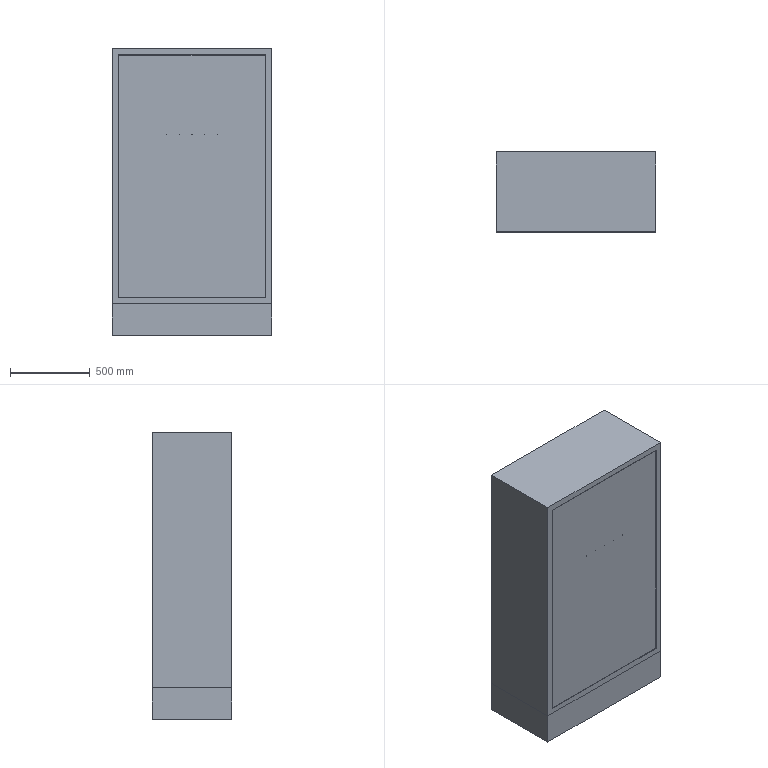Part | NX | features BREP 2 | 2 solids | 42 faces | box 1000 x 500 x 1800 mm | volume 899902130 mm3 | plane 22 | cylinder 10 | cone 10 | commonest cylinder face diameters 2 x10
STEP:
#1=CARTESIAN_POINT('',(500.,-250.,0.));
#2=VERTEX_POINT('',#1);
#3=CARTESIAN_POINT('',(500.,250.,0.));
#4=VERTEX_POINT('',#3);
#5=CARTESIAN_POINT('',(500.,-250.,0.));
#6=DIRECTION('',(0.,1.,0.));
#7=VECTOR('',#6,1000.);
#8=LINE('',#5,#7);
#9=EDGE_CURVE('',#2,#4,#8,.T.);
#10=ORIENTED_EDGE('',*,*,#9,.T.);
#11=CARTESIAN_POINT('',(500.,250.,200.));
#12=VERTEX_POINT('',#11);
#13=CARTESIAN_POINT('',(500.,250.,200.));
#14=DIRECTION('',(0.,0.,-1.));
#15=VECTOR('',#14,1000.);
#16=LINE('',#13,#15);
#17=EDGE_CURVE('',#12,#4,#16,.T.);
#18=ORIENTED_EDGE('',*,*,#17,.F.);
#19=CARTESIAN_POINT('',(500.,-250.,200.));
#20=VERTEX_POINT('',#19);
#21=CARTESIAN_POINT('',(500.,-250.,200.));
#22=DIRECTION('',(0.,1.,0.));
#23=VECTOR('',#22,1000.);
#24=LINE('',#21,#23);
#25=EDGE_CURVE('',#20,#12,#24,.T.);
#26=ORIENTED_EDGE('',*,*,#25,.F.);
#27=CARTESIAN_POINT('',(500.,-250.,200.));
#28=DIRECTION('',(0.,0.,-1.));
#29=VECTOR('',#28,1000.);
#30=LINE('',#27,#29);
#31=EDGE_CURVE('',#20,#2,#30,.T.);
#32=ORIENTED_EDGE('',*,*,#31,.T.);
#33=EDGE_LOOP('',(#10,#18,#26,#32));
#34=FACE_BOUND('',#33,.T.);
#35=CARTESIAN_POINT('',(500.,-250.,200.));
#36=DIRECTION('',(-1.,0.,0.));
#37=DIRECTION('',(0.,0.,1.));
#38=AXIS2_PLACEMENT_3D('',#35,#36,#37);
#39=PLANE('',#38);
#40=ADVANCED_FACE('',(#34),#39,.F.);
#41=CARTESIAN_POINT('',(-500.,250.,0.));
#42=VERTEX_POINT('',#41);
#43=CARTESIAN_POINT('',(-500.,250.,0.));
#44=DIRECTION('',(-1.,0.,0.));
#45=VECTOR('',#44,1000.);
#46=LINE('',#43,#45);
#47=EDGE_CURVE('',#4,#42,#46,.T.);
#48=ORIENTED_EDGE('',*,*,#47,.T.);
#49=CARTESIAN_POINT('',(-500.,250.,200.));
#50=VERTEX_POINT('',#49);
#51=CARTESIAN_POINT('',(-500.,250.,200.));
#52=DIRECTION('',(0.,0.,-1.));
#53=VECTOR('',#52,1000.);
#54=LINE('',#51,#53);
#55=EDGE_CURVE('',#50,#42,#54,.T.);
#56=ORIENTED_EDGE('',*,*,#55,.F.);
#57=CARTESIAN_POINT('',(-500.,250.,200.));
#58=DIRECTION('',(-1.,0.,0.));
#59=VECTOR('',#58,1000.);
#60=LINE('',#57,#59);
#61=EDGE_CURVE('',#12,#50,#60,.T.);
#62=ORIENTED_EDGE('',*,*,#61,.F.);
#63=ORIENTED_EDGE('',*,*,#17,.T.);
#64=EDGE_LOOP('',(#48,#56,#62,#63));
#65=FACE_BOUND('',#64,.T.);
#66=CARTESIAN_POINT('',(-500.,250.,200.));
#67=DIRECTION('',(0.,-1.,0.));
#68=DIRECTION('',(0.,0.,-1.));
#69=AXIS2_PLACEMENT_3D('',#66,#67,#68);
#70=PLANE('',#69);
#71=ADVANCED_FACE('',(#65),#70,.F.);
#72=CARTESIAN_POINT('',(-500.,-250.,0.));
#73=VERTEX_POINT('',#72);
#74=CARTESIAN_POINT('',(-500.,-250.,0.));
#75=DIRECTION('',(0.,-1.,0.));
#76=VECTOR('',#75,1000.);
#77=LINE('',#74,#76);
#78=EDGE_CURVE('',#42,#73,#77,.T.);
#79=ORIENTED_EDGE('',*,*,#78,.T.);
#80=CARTESIAN_POINT('',(-500.,-250.,200.));
#81=VERTEX_POINT('',#80);
#82=CARTESIAN_POINT('',(-500.,-250.,200.));
#83=DIRECTION('',(0.,0.,-1.));
#84=VECTOR('',#83,1000.);
#85=LINE('',#82,#84);
#86=EDGE_CURVE('',#81,#73,#85,.T.);
#87=ORIENTED_EDGE('',*,*,#86,.F.);
#88=CARTESIAN_POINT('',(-500.,-250.,200.));
#89=DIRECTION('',(0.,-1.,0.));
#90=VECTOR('',#89,1000.);
#91=LINE('',#88,#90);
#92=EDGE_CURVE('',#50,#81,#91,.T.);
#93=ORIENTED_EDGE('',*,*,#92,.F.);
#94=ORIENTED_EDGE('',*,*,#55,.T.);
#95=EDGE_LOOP('',(#79,#87,#93,#94));
#96=FACE_BOUND('',#95,.T.);
#97=CARTESIAN_POINT('',(-500.,-250.,200.));
#98=DIRECTION('',(1.,0.,0.));
#99=DIRECTION('',(0.,1.,0.));
#100=AXIS2_PLACEMENT_3D('',#97,#98,#99);
#101=PLANE('',#100);
#102=ADVANCED_FACE('',(#96),#101,.F.);
#103=CARTESIAN_POINT('',(-500.,-250.,0.));
#104=DIRECTION('',(1.,0.,0.));
#105=VECTOR('',#104,1000.);
#106=LINE('',#103,#105);
#107=EDGE_CURVE('',#73,#2,#106,.T.);
#108=ORIENTED_EDGE('',*,*,#107,.T.);
#109=ORIENTED_EDGE('',*,*,#31,.F.);
#110=CARTESIAN_POINT('',(-500.,-250.,200.));
#111=DIRECTION('',(1.,0.,0.));
#112=VECTOR('',#111,1000.);
#113=LINE('',#110,#112);
#114=EDGE_CURVE('',#81,#20,#113,.T.);
#115=ORIENTED_EDGE('',*,*,#114,.F.);
#116=ORIENTED_EDGE('',*,*,#86,.T.);
#117=EDGE_LOOP('',(#108,#109,#115,#116));
#118=FACE_BOUND('',#117,.T.);
#119=CARTESIAN_POINT('',(-500.,-250.,200.));
#120=DIRECTION('',(0.,1.,0.));
#121=DIRECTION('',(1.,0.,0.));
#122=AXIS2_PLACEMENT_3D('',#119,#120,#121);
#123=PLANE('',#122);
#124=ADVANCED_FACE('',(#118),#123,.F.);
#125=ORIENTED_EDGE('',*,*,#25,.T.);
#126=ORIENTED_EDGE('',*,*,#61,.T.);
#127=ORIENTED_EDGE('',*,*,#92,.T.);
#128=ORIENTED_EDGE('',*,*,#114,.T.);
#129=EDGE_LOOP('',(#125,#126,#127,#128));
#130=FACE_BOUND('',#129,.T.);
#131=CARTESIAN_POINT('',(0.,0.,200.));
#132=DIRECTION('',(0.,0.,-1.));
#133=DIRECTION('',(0.,-1.,0.));
#134=AXIS2_PLACEMENT_3D('',#131,#132,#133);
#135=PLANE('',#134);
#136=ADVANCED_FACE('',(#130),#135,.F.);
#137=ORIENTED_EDGE('',*,*,#9,.F.);
#138=ORIENTED_EDGE('',*,*,#107,.F.);
#139=ORIENTED_EDGE('',*,*,#78,.F.);
#140=ORIENTED_EDGE('',*,*,#47,.F.);
#141=EDGE_LOOP('',(#137,#138,#139,#140));
#142=FACE_BOUND('',#141,.T.);
#143=CARTESIAN_POINT('',(0.,0.,0.));
#144=DIRECTION('',(0.,0.,-1.));
#145=DIRECTION('',(0.,-1.,0.));
#146=AXIS2_PLACEMENT_3D('',#143,#144,#145);
#147=PLANE('',#146);
#148=ADVANCED_FACE('',(#142),#147,.T.);
#149=CLOSED_SHELL('',(#40,#71,#102,#124,#136,#148));
#150=MANIFOLD_SOLID_BREP('',#149);
#151=CARTESIAN_POINT('',(-160.,-233.,1260.));
#152=VERTEX_POINT('',#151);
#153=CARTESIAN_POINT('',(-160.,-233.,1258.));
#154=VERTEX_POINT('',#153);
#155=CARTESIAN_POINT('',(-160.,-233.,1259.));
#156=DIRECTION('',(0.,-1.,0.));
#157=DIRECTION('',(0.,0.,-1.));
#158=AXIS2_PLACEMENT_3D('',#155,#156,#157);
#159=CIRCLE('',#158,1.);
#160=EDGE_CURVE('',#152,#154,#159,.T.);
#161=ORIENTED_EDGE('',*,*,#160,.F.);
#162=CARTESIAN_POINT('',(-160.,-250.,1260.));
#163=VERTEX_POINT('',#162);
#164=CARTESIAN_POINT('',(-160.,-250.,1260.));
#165=DIRECTION('',(0.,-1.,0.));
#166=VECTOR('',#165,1000.);
#167=LINE('',#164,#166);
#168=EDGE_CURVE('',#152,#163,#167,.T.);
#169=ORIENTED_EDGE('',*,*,#168,.T.);
#170=CARTESIAN_POINT('',(-160.,-250.,1258.));
#171=VERTEX_POINT('',#170);
#172=CARTESIAN_POINT('',(-160.,-250.,1259.));
#173=DIRECTION('',(0.,-1.,0.));
#174=DIRECTION('',(0.,0.,-1.));
#175=AXIS2_PLACEMENT_3D('',#172,#173,#174);
#176=CIRCLE('',#175,1.);
#177=EDGE_CURVE('',#163,#171,#176,.T.);
#178=ORIENTED_EDGE('',*,*,#177,.T.);
#179=CARTESIAN_POINT('',(-160.,-250.,1258.));
#180=DIRECTION('',(0.,-1.,0.));
#181=VECTOR('',#180,1000.);
#182=LINE('',#179,#181);
#183=EDGE_CURVE('',#154,#171,#182,.T.);
#184=ORIENTED_EDGE('',*,*,#183,.F.);
#185=EDGE_LOOP('',(#161,#169,#178,#184));
#186=FACE_BOUND('',#185,.T.);
#187=CARTESIAN_POINT('',(-160.,-250.,1259.));
#188=DIRECTION('',(0.,-1.,0.));
#189=DIRECTION('',(0.,0.,-1.));
#190=AXIS2_PLACEMENT_3D('',#187,#188,#189);
#191=CYLINDRICAL_SURFACE('',#190,1.);
#192=ADVANCED_FACE('',(#186),#191,.F.);
#193=CARTESIAN_POINT('',(-160.,-232.399,1259.));
#194=VERTEX_POINT('',#193);
#195=CARTESIAN_POINT('',(-160.,-233.,1258.));
#196=DIRECTION('',(0.,-0.515,-0.8572));
#197=VECTOR('',#196,1000.);
#198=LINE('',#195,#197);
#199=EDGE_CURVE('',#194,#154,#198,.T.);
#200=ORIENTED_EDGE('',*,*,#199,.F.);
#201=CARTESIAN_POINT('',(-160.,-233.,1260.));
#202=DIRECTION('',(0.,-0.515,0.8572));
#203=VECTOR('',#202,1000.);
#204=LINE('',#201,#203);
#205=EDGE_CURVE('',#194,#152,#204,.T.);
#206=ORIENTED_EDGE('',*,*,#205,.T.);
#207=ORIENTED_EDGE('',*,*,#160,.T.);
#208=EDGE_LOOP('',(#200,#206,#207));
#209=FACE_BOUND('',#208,.T.);
#210=CARTESIAN_POINT('',(-160.,-233.,1259.));
#211=DIRECTION('',(0.,-1.,0.));
#212=DIRECTION('',(0.,0.,-1.));
#213=AXIS2_PLACEMENT_3D('',#210,#211,#212);
#214=CONICAL_SURFACE('',#213,1.,1.03);
#215=ADVANCED_FACE('',(#209),#214,.F.);
#216=CARTESIAN_POINT('',(-80.,-233.,1260.));
#217=VERTEX_POINT('',#216);
#218=CARTESIAN_POINT('',(-80.,-233.,1258.));
#219=VERTEX_POINT('',#218);
#220=CARTESIAN_POINT('',(-80.,-233.,1259.));
#221=DIRECTION('',(0.,-1.,0.));
#222=DIRECTION('',(0.,0.,-1.));
#223=AXIS2_PLACEMENT_3D('',#220,#221,#222);
#224=CIRCLE('',#223,1.);
#225=EDGE_CURVE('',#217,#219,#224,.T.);
#226=ORIENTED_EDGE('',*,*,#225,.F.);
#227=CARTESIAN_POINT('',(-80.,-250.,1260.));
#228=VERTEX_POINT('',#227);
#229=CARTESIAN_POINT('',(-80.,-250.,1260.));
#230=DIRECTION('',(0.,-1.,0.));
#231=VECTOR('',#230,1000.);
#232=LINE('',#229,#231);
#233=EDGE_CURVE('',#217,#228,#232,.T.);
#234=ORIENTED_EDGE('',*,*,#233,.T.);
#235=CARTESIAN_POINT('',(-80.,-250.,1258.));
#236=VERTEX_POINT('',#235);
#237=CARTESIAN_POINT('',(-80.,-250.,1259.));
#238=DIRECTION('',(0.,-1.,0.));
#239=DIRECTION('',(0.,0.,-1.));
#240=AXIS2_PLACEMENT_3D('',#237,#238,#239);
#241=CIRCLE('',#240,1.);
#242=EDGE_CURVE('',#228,#236,#241,.T.);
#243=ORIENTED_EDGE('',*,*,#242,.T.);
#244=CARTESIAN_POINT('',(-80.,-250.,1258.));
#245=DIRECTION('',(0.,-1.,0.));
#246=VECTOR('',#245,1000.);
#247=LINE('',#244,#246);
#248=EDGE_CURVE('',#219,#236,#247,.T.);
#249=ORIENTED_EDGE('',*,*,#248,.F.);
#250=EDGE_LOOP('',(#226,#234,#243,#249));
#251=FACE_BOUND('',#250,.T.);
#252=CARTESIAN_POINT('',(-80.,-250.,1259.));
#253=DIRECTION('',(0.,-1.,0.));
#254=DIRECTION('',(0.,0.,-1.));
#255=AXIS2_PLACEMENT_3D('',#252,#253,#254);
#256=CYLINDRICAL_SURFACE('',#255,1.);
#257=ADVANCED_FACE('',(#251),#256,.F.);
#258=CARTESIAN_POINT('',(-80.,-232.399,1259.));
#259=VERTEX_POINT('',#258);
#260=CARTESIAN_POINT('',(-80.,-233.,1258.));
#261=DIRECTION('',(0.,-0.515,-0.8572));
#262=VECTOR('',#261,1000.);
#263=LINE('',#260,#262);
#264=EDGE_CURVE('',#259,#219,#263,.T.);
#265=ORIENTED_EDGE('',*,*,#264,.F.);
#266=CARTESIAN_POINT('',(-80.,-233.,1260.));
#267=DIRECTION('',(0.,-0.515,0.8572));
#268=VECTOR('',#267,1000.);
#269=LINE('',#266,#268);
#270=EDGE_CURVE('',#259,#217,#269,.T.);
#271=ORIENTED_EDGE('',*,*,#270,.T.);
#272=ORIENTED_EDGE('',*,*,#225,.T.);
#273=EDGE_LOOP('',(#265,#271,#272));
#274=FACE_BOUND('',#273,.T.);
#275=CARTESIAN_POINT('',(-80.,-233.,1259.));
#276=DIRECTION('',(0.,-1.,0.));
#277=DIRECTION('',(0.,0.,-1.));
#278=AXIS2_PLACEMENT_3D('',#275,#276,#277);
#279=CONICAL_SURFACE('',#278,1.,1.03);
#280=ADVANCED_FACE('',(#274),#279,.F.);
#281=CARTESIAN_POINT('',(0.,-233.,1260.));
#282=VERTEX_POINT('',#281);
#283=CARTESIAN_POINT('',(0.,-233.,1258.));
#284=VERTEX_POINT('',#283);
#285=CARTESIAN_POINT('',(0.,-233.,1259.));
#286=DIRECTION('',(0.,-1.,0.));
#287=DIRECTION('',(0.,0.,-1.));
#288=AXIS2_PLACEMENT_3D('',#285,#286,#287);
#289=CIRCLE('',#288,1.);
#290=EDGE_CURVE('',#282,#284,#289,.T.);
#291=ORIENTED_EDGE('',*,*,#290,.F.);
#292=CARTESIAN_POINT('',(0.,-250.,1260.));
#293=VERTEX_POINT('',#292);
#294=CARTESIAN_POINT('',(0.,-250.,1260.));
#295=DIRECTION('',(0.,-1.,0.));
#296=VECTOR('',#295,1000.);
#297=LINE('',#294,#296);
#298=EDGE_CURVE('',#282,#293,#297,.T.);
#299=ORIENTED_EDGE('',*,*,#298,.T.);
#300=CARTESIAN_POINT('',(0.,-250.,1258.));
#301=VERTEX_POINT('',#300);
#302=CARTESIAN_POINT('',(0.,-250.,1259.));
#303=DIRECTION('',(0.,-1.,0.));
#304=DIRECTION('',(0.,0.,-1.));
#305=AXIS2_PLACEMENT_3D('',#302,#303,#304);
#306=CIRCLE('',#305,1.);
#307=EDGE_CURVE('',#293,#301,#306,.T.);
#308=ORIENTED_EDGE('',*,*,#307,.T.);
#309=CARTESIAN_POINT('',(0.,-250.,1258.));
#310=DIRECTION('',(0.,-1.,0.));
#311=VECTOR('',#310,1000.);
#312=LINE('',#309,#311);
#313=EDGE_CURVE('',#284,#301,#312,.T.);
#314=ORIENTED_EDGE('',*,*,#313,.F.);
#315=EDGE_LOOP('',(#291,#299,#308,#314));
#316=FACE_BOUND('',#315,.T.);
#317=CARTESIAN_POINT('',(0.,-250.,1259.));
#318=DIRECTION('',(0.,-1.,0.));
#319=DIRECTION('',(0.,0.,-1.));
#320=AXIS2_PLACEMENT_3D('',#317,#318,#319);
#321=CYLINDRICAL_SURFACE('',#320,1.);
#322=ADVANCED_FACE('',(#316),#321,.F.);
#323=CARTESIAN_POINT('',(0.,-232.399,1259.));
#324=VERTEX_POINT('',#323);
#325=CARTESIAN_POINT('',(0.,-233.,1258.));
#326=DIRECTION('',(0.,-0.515,-0.8572));
#327=VECTOR('',#326,1000.);
#328=LINE('',#325,#327);
#329=EDGE_CURVE('',#324,#284,#328,.T.);
#330=ORIENTED_EDGE('',*,*,#329,.F.);
#331=CARTESIAN_POINT('',(0.,-233.,1260.));
#332=DIRECTION('',(0.,-0.515,0.8572));
#333=VECTOR('',#332,1000.);
#334=LINE('',#331,#333);
#335=EDGE_CURVE('',#324,#282,#334,.T.);
#336=ORIENTED_EDGE('',*,*,#335,.T.);
#337=ORIENTED_EDGE('',*,*,#290,.T.);
#338=EDGE_LOOP('',(#330,#336,#337));
#339=FACE_BOUND('',#338,.T.);
#340=CARTESIAN_POINT('',(0.,-233.,1259.));
#341=DIRECTION('',(0.,-1.,0.));
#342=DIRECTION('',(0.,0.,-1.));
#343=AXIS2_PLACEMENT_3D('',#340,#341,#342);
#344=CONICAL_SURFACE('',#343,1.,1.03);
#345=ADVANCED_FACE('',(#339),#344,.F.);
#346=CARTESIAN_POINT('',(80.,-233.,1260.));
#347=VERTEX_POINT('',#346);
#348=CARTESIAN_POINT('',(80.,-233.,1258.));
#349=VERTEX_POINT('',#348);
#350=CARTESIAN_POINT('',(80.,-233.,1259.));
#351=DIRECTION('',(0.,-1.,0.));
#352=DIRECTION('',(0.,0.,-1.));
#353=AXIS2_PLACEMENT_3D('',#350,#351,#352);
#354=CIRCLE('',#353,1.);
#355=EDGE_CURVE('',#347,#349,#354,.T.);
#356=ORIENTED_EDGE('',*,*,#355,.F.);
#357=CARTESIAN_POINT('',(80.,-250.,1260.));
#358=VERTEX_POINT('',#357);
#359=CARTESIAN_POINT('',(80.,-250.,1260.));
#360=DIRECTION('',(0.,-1.,0.));
#361=VECTOR('',#360,1000.);
#362=LINE('',#359,#361);
#363=EDGE_CURVE('',#347,#358,#362,.T.);
#364=ORIENTED_EDGE('',*,*,#363,.T.);
#365=CARTESIAN_POINT('',(80.,-250.,1258.));
#366=VERTEX_POINT('',#365);
#367=CARTESIAN_POINT('',(80.,-250.,1259.));
#368=DIRECTION('',(0.,-1.,0.));
#369=DIRECTION('',(0.,0.,-1.));
#370=AXIS2_PLACEMENT_3D('',#367,#368,#369);
#371=CIRCLE('',#370,1.);
#372=EDGE_CURVE('',#358,#366,#371,.T.);
#373=ORIENTED_EDGE('',*,*,#372,.T.);
#374=CARTESIAN_POINT('',(80.,-250.,1258.));
#375=DIRECTION('',(0.,-1.,0.));
#376=VECTOR('',#375,1000.);
#377=LINE('',#374,#376);
#378=EDGE_CURVE('',#349,#366,#377,.T.);
#379=ORIENTED_EDGE('',*,*,#378,.F.);
#380=EDGE_LOOP('',(#356,#364,#373,#379));
#381=FACE_BOUND('',#380,.T.);
#382=CARTESIAN_POINT('',(80.,-250.,1259.));
#383=DIRECTION('',(0.,-1.,0.));
#384=DIRECTION('',(0.,0.,-1.));
#385=AXIS2_PLACEMENT_3D('',#382,#383,#384);
#386=CYLINDRICAL_SURFACE('',#385,1.);
#387=ADVANCED_FACE('',(#381),#386,.F.);
#388=CARTESIAN_POINT('',(80.,-232.399,1259.));
#389=VERTEX_POINT('',#388);
#390=CARTESIAN_POINT('',(80.,-233.,1258.));
#391=DIRECTION('',(0.,-0.515,-0.8572));
#392=VECTOR('',#391,1000.);
#393=LINE('',#390,#392);
#394=EDGE_CURVE('',#389,#349,#393,.T.);
#395=ORIENTED_EDGE('',*,*,#394,.F.);
#396=CARTESIAN_POINT('',(80.,-233.,1260.));
#397=DIRECTION('',(0.,-0.515,0.8572));
#398=VECTOR('',#397,1000.);
#399=LINE('',#396,#398);
#400=EDGE_CURVE('',#389,#347,#399,.T.);
#401=ORIENTED_EDGE('',*,*,#400,.T.);
#402=ORIENTED_EDGE('',*,*,#355,.T.);
#403=EDGE_LOOP('',(#395,#401,#402));
#404=FACE_BOUND('',#403,.T.);
#405=CARTESIAN_POINT('',(80.,-233.,1259.));
#406=DIRECTION('',(0.,-1.,0.));
#407=DIRECTION('',(0.,0.,-1.));
#408=AXIS2_PLACEMENT_3D('',#405,#406,#407);
#409=CONICAL_SURFACE('',#408,1.,1.03);
#410=ADVANCED_FACE('',(#404),#409,.F.);
#411=CARTESIAN_POINT('',(160.,-233.,1260.));
#412=VERTEX_POINT('',#411);
#413=CARTESIAN_POINT('',(160.,-233.,1258.));
#414=VERTEX_POINT('',#413);
#415=CARTESIAN_POINT('',(160.,-233.,1259.));
#416=DIRECTION('',(0.,-1.,0.));
#417=DIRECTION('',(0.,0.,-1.));
#418=AXIS2_PLACEMENT_3D('',#415,#416,#417);
#419=CIRCLE('',#418,1.);
#420=EDGE_CURVE('',#412,#414,#419,.T.);
#421=ORIENTED_EDGE('',*,*,#420,.F.);
#422=CARTESIAN_POINT('',(160.,-250.,1260.));
#423=VERTEX_POINT('',#422);
#424=CARTESIAN_POINT('',(160.,-250.,1260.));
#425=DIRECTION('',(0.,-1.,0.));
#426=VECTOR('',#425,1000.);
#427=LINE('',#424,#426);
#428=EDGE_CURVE('',#412,#423,#427,.T.);
#429=ORIENTED_EDGE('',*,*,#428,.T.);
#430=CARTESIAN_POINT('',(160.,-250.,1258.));
#431=VERTEX_POINT('',#430);
#432=CARTESIAN_POINT('',(160.,-250.,1259.));
#433=DIRECTION('',(0.,-1.,0.));
#434=DIRECTION('',(0.,0.,-1.));
#435=AXIS2_PLACEMENT_3D('',#432,#433,#434);
#436=CIRCLE('',#435,1.);
#437=EDGE_CURVE('',#423,#431,#436,.T.);
#438=ORIENTED_EDGE('',*,*,#437,.T.);
#439=CARTESIAN_POINT('',(160.,-250.,1258.));
#440=DIRECTION('',(0.,-1.,0.));
#441=VECTOR('',#440,1000.);
#442=LINE('',#439,#441);
#443=EDGE_CURVE('',#414,#431,#442,.T.);
#444=ORIENTED_EDGE('',*,*,#443,.F.);
#445=EDGE_LOOP('',(#421,#429,#438,#444));
#446=FACE_BOUND('',#445,.T.);
#447=CARTESIAN_POINT('',(160.,-250.,1259.));
#448=DIRECTION('',(0.,-1.,0.));
#449=DIRECTION('',(0.,0.,-1.));
#450=AXIS2_PLACEMENT_3D('',#447,#448,#449);
#451=CYLINDRICAL_SURFACE('',#450,1.);
#452=ADVANCED_FACE('',(#446),#451,.F.);
#453=CARTESIAN_POINT('',(160.,-232.399,1259.));
#454=VERTEX_POINT('',#453);
#455=CARTESIAN_POINT('',(160.,-233.,1258.));
#456=DIRECTION('',(0.,-0.515,-0.8572));
#457=VECTOR('',#456,1000.);
#458=LINE('',#455,#457);
#459=EDGE_CURVE('',#454,#414,#458,.T.);
#460=ORIENTED_EDGE('',*,*,#459,.F.);
#461=CARTESIAN_POINT('',(160.,-233.,1260.));
#462=DIRECTION('',(0.,-0.515,0.8572));
#463=VECTOR('',#462,1000.);
#464=LINE('',#461,#463);
#465=EDGE_CURVE('',#454,#412,#464,.T.);
#466=ORIENTED_EDGE('',*,*,#465,.T.);
#467=ORIENTED_EDGE('',*,*,#420,.T.);
#468=EDGE_LOOP('',(#460,#466,#467));
#469=FACE_BOUND('',#468,.T.);
#470=CARTESIAN_POINT('',(160.,-233.,1259.));
#471=DIRECTION('',(0.,-1.,0.));
#472=DIRECTION('',(0.,0.,-1.));
#473=AXIS2_PLACEMENT_3D('',#470,#471,#472);
#474=CONICAL_SURFACE('',#473,1.,1.03);
#475=ADVANCED_FACE('',(#469),#474,.F.);
#476=CARTESIAN_POINT('',(-459.,-250.,1759.));
#477=VERTEX_POINT('',#476);
#478=CARTESIAN_POINT('',(-459.,-250.,241.));
#479=VERTEX_POINT('',#478);
#480=CARTESIAN_POINT('',(-459.,-250.,1760.));
#481=DIRECTION('',(0.,0.,-1.));
#482=VECTOR('',#481,1000.);
#483=LINE('',#480,#482);
#484=EDGE_CURVE('',#477,#479,#483,.T.);
#485=ORIENTED_EDGE('',*,*,#484,.T.);
#486=CARTESIAN_POINT('',(459.,-250.,241.));
#487=VERTEX_POINT('',#486);
#488=CARTESIAN_POINT('',(-460.,-250.,241.));
#489=DIRECTION('',(1.,0.,0.));
#490=VECTOR('',#489,1000.);
#491=LINE('',#488,#490);
#492=EDGE_CURVE('',#479,#487,#491,.T.);
#493=ORIENTED_EDGE('',*,*,#492,.T.);
#494=CARTESIAN_POINT('',(459.,-250.,1759.));
#495=VERTEX_POINT('',#494);
#496=CARTESIAN_POINT('',(459.,-250.,240.));
#497=DIRECTION('',(0.,0.,1.));
#498=VECTOR('',#497,1000.);
#499=LINE('',#496,#498);
#500=EDGE_CURVE('',#487,#495,#499,.T.);
#501=ORIENTED_EDGE('',*,*,#500,.T.);
#502=CARTESIAN_POINT('',(460.,-250.,1759.));
#503=DIRECTION('',(-1.,0.,0.));
#504=VECTOR('',#503,1000.);
#505=LINE('',#502,#504);
#506=EDGE_CURVE('',#495,#477,#505,.T.);
#507=ORIENTED_EDGE('',*,*,#506,.T.);
#508=EDGE_LOOP('',(#485,#493,#501,#507));
#509=FACE_BOUND('',#508,.T.);
#510=CARTESIAN_POINT('',(-160.,-250.,1259.));
#511=DIRECTION('',(0.,-1.,0.));
#512=DIRECTION('',(0.,0.,-1.));
#513=AXIS2_PLACEMENT_3D('',#510,#511,#512);
#514=CIRCLE('',#513,1.);
#515=EDGE_CURVE('',#171,#163,#514,.T.);
#516=ORIENTED_EDGE('',*,*,#515,.F.);
#517=ORIENTED_EDGE('',*,*,#177,.F.);
#518=EDGE_LOOP('',(#516,#517));
#519=FACE_BOUND('',#518,.T.);
#520=CARTESIAN_POINT('',(-80.,-250.,1259.));
#521=DIRECTION('',(0.,-1.,0.));
#522=DIRECTION('',(0.,0.,-1.));
#523=AXIS2_PLACEMENT_3D('',#520,#521,#522);
#524=CIRCLE('',#523,1.);
#525=EDGE_CURVE('',#236,#228,#524,.T.);
#526=ORIENTED_EDGE('',*,*,#525,.F.);
#527=ORIENTED_EDGE('',*,*,#242,.F.);
#528=EDGE_LOOP('',(#526,#527));
#529=FACE_BOUND('',#528,.T.);
#530=CARTESIAN_POINT('',(0.,-250.,1259.));
#531=DIRECTION('',(0.,-1.,0.));
#532=DIRECTION('',(0.,0.,-1.));
#533=AXIS2_PLACEMENT_3D('',#530,#531,#532);
#534=CIRCLE('',#533,1.);
#535=EDGE_CURVE('',#301,#293,#534,.T.);
#536=ORIENTED_EDGE('',*,*,#535,.F.);
#537=ORIENTED_EDGE('',*,*,#307,.F.);
#538=EDGE_LOOP('',(#536,#537));
#539=FACE_BOUND('',#538,.T.);
#540=CARTESIAN_POINT('',(160.,-250.,1259.));
#541=DIRECTION('',(0.,-1.,0.));
#542=DIRECTION('',(0.,0.,-1.));
#543=AXIS2_PLACEMENT_3D('',#540,#541,#542);
#544=CIRCLE('',#543,1.);
#545=EDGE_CURVE('',#431,#423,#544,.T.);
#546=ORIENTED_EDGE('',*,*,#545,.F.);
#547=ORIENTED_EDGE('',*,*,#437,.F.);
#548=EDGE_LOOP('',(#546,#547));
#549=FACE_BOUND('',#548,.T.);
#550=CARTESIAN_POINT('',(80.,-250.,1259.));
#551=DIRECTION('',(0.,-1.,0.));
#552=DIRECTION('',(0.,0.,-1.));
#553=AXIS2_PLACEMENT_3D('',#550,#551,#552);
#554=CIRCLE('',#553,1.);
#555=EDGE_CURVE('',#366,#358,#554,.T.);
#556=ORIENTED_EDGE('',*,*,#555,.F.);
#557=ORIENTED_EDGE('',*,*,#372,.F.);
#558=EDGE_LOOP('',(#556,#557));
#559=FACE_BOUND('',#558,.T.);
#560=CARTESIAN_POINT('',(-500.,-250.,1800.));
#561=DIRECTION('',(0.,1.,0.));
#562=DIRECTION('',(1.,0.,0.));
#563=AXIS2_PLACEMENT_3D('',#560,#561,#562);
#564=PLANE('',#563);
#565=ADVANCED_FACE('',(#509,#519,#529,#539,#549,#559),#564,.F.);
#566=CARTESIAN_POINT('',(-500.,-250.,200.));
#567=VERTEX_POINT('',#566);
#568=CARTESIAN_POINT('',(500.,-250.,200.));
#569=VERTEX_POINT('',#568);
#570=CARTESIAN_POINT('',(-500.,-250.,200.));
#571=DIRECTION('',(1.,0.,0.));
#572=VECTOR('',#571,1000.);
#573=LINE('',#570,#572);
#574=EDGE_CURVE('',#567,#569,#573,.T.);
#575=ORIENTED_EDGE('',*,*,#574,.T.);
#576=CARTESIAN_POINT('',(500.,-250.,1800.));
#577=VERTEX_POINT('',#576);
#578=CARTESIAN_POINT('',(500.,-250.,1800.));
#579=DIRECTION('',(0.,0.,-1.));
#580=VECTOR('',#579,1000.);
#581=LINE('',#578,#580);
#582=EDGE_CURVE('',#577,#569,#581,.T.);
#583=ORIENTED_EDGE('',*,*,#582,.F.);
#584=CARTESIAN_POINT('',(-500.,-250.,1800.));
#585=VERTEX_POINT('',#584);
#586=CARTESIAN_POINT('',(-500.,-250.,1800.));
#587=DIRECTION('',(1.,0.,0.));
#588=VECTOR('',#587,1000.);
#589=LINE('',#586,#588);
#590=EDGE_CURVE('',#585,#577,#589,.T.);
#591=ORIENTED_EDGE('',*,*,#590,.F.);
#592=CARTESIAN_POINT('',(-500.,-250.,1800.));
#593=DIRECTION('',(0.,0.,-1.));
#594=VECTOR('',#593,1000.);
#595=LINE('',#592,#594);
#596=EDGE_CURVE('',#585,#567,#595,.T.);
#597=ORIENTED_EDGE('',*,*,#596,.T.);
#598=EDGE_LOOP('',(#575,#583,#591,#597));
#599=FACE_BOUND('',#598,.T.);
#600=CARTESIAN_POINT('',(-461.,-250.,239.));
#601=VERTEX_POINT('',#600);
#602=CARTESIAN_POINT('',(461.,-250.,239.));
#603=VERTEX_POINT('',#602);
#604=CARTESIAN_POINT('',(-460.,-250.,239.));
#605=DIRECTION('',(1.,0.,0.));
#606=VECTOR('',#605,1000.);
#607=LINE('',#604,#606);
#608=EDGE_CURVE('',#601,#603,#607,.T.);
#609=ORIENTED_EDGE('',*,*,#608,.F.);
#610=CARTESIAN_POINT('',(-461.,-250.,1761.));
#611=VERTEX_POINT('',#610);
#612=CARTESIAN_POINT('',(-461.,-250.,1760.));
#613=DIRECTION('',(0.,0.,-1.));
#614=VECTOR('',#613,1000.);
#615=LINE('',#612,#614);
#616=EDGE_CURVE('',#611,#601,#615,.T.);
#617=ORIENTED_EDGE('',*,*,#616,.F.);
#618=CARTESIAN_POINT('',(461.,-250.,1761.));
#619=VERTEX_POINT('',#618);
#620=CARTESIAN_POINT('',(460.,-250.,1761.));
#621=DIRECTION('',(-1.,0.,0.));
#622=VECTOR('',#621,1000.);
#623=LINE('',#620,#622);
#624=EDGE_CURVE('',#619,#611,#623,.T.);
#625=ORIENTED_EDGE('',*,*,#624,.F.);
#626=CARTESIAN_POINT('',(461.,-250.,240.));
#627=DIRECTION('',(0.,0.,1.));
#628=VECTOR('',#627,1000.);
#629=LINE('',#626,#628);
#630=EDGE_CURVE('',#603,#619,#629,.T.);
#631=ORIENTED_EDGE('',*,*,#630,.F.);
#632=EDGE_LOOP('',(#609,#617,#625,#631));
#633=FACE_BOUND('',#632,.T.);
#634=CARTESIAN_POINT('',(-500.,-250.,1800.));
#635=DIRECTION('',(0.,1.,0.));
#636=DIRECTION('',(1.,0.,0.));
#637=AXIS2_PLACEMENT_3D('',#634,#635,#636);
#638=PLANE('',#637);
#639=ADVANCED_FACE('',(#599,#633),#638,.F.);
#640=CARTESIAN_POINT('',(500.,250.,200.));
#641=VERTEX_POINT('',#640);
#642=CARTESIAN_POINT('',(500.,-250.,200.));
#643=DIRECTION('',(0.,1.,0.));
#644=VECTOR('',#643,1000.);
#645=LINE('',#642,#644);
#646=EDGE_CURVE('',#569,#641,#645,.T.);
#647=ORIENTED_EDGE('',*,*,#646,.T.);
#648=CARTESIAN_POINT('',(500.,250.,1800.));
#649=VERTEX_POINT('',#648);
#650=CARTESIAN_POINT('',(500.,250.,1800.));
#651=DIRECTION('',(0.,0.,-1.));
#652=VECTOR('',#651,1000.);
#653=LINE('',#650,#652);
#654=EDGE_CURVE('',#649,#641,#653,.T.);
#655=ORIENTED_EDGE('',*,*,#654,.F.);
#656=CARTESIAN_POINT('',(500.,-250.,1800.));
#657=DIRECTION('',(0.,1.,0.));
#658=VECTOR('',#657,1000.);
#659=LINE('',#656,#658);
#660=EDGE_CURVE('',#577,#649,#659,.T.);
#661=ORIENTED_EDGE('',*,*,#660,.F.);
#662=ORIENTED_EDGE('',*,*,#582,.T.);
#663=EDGE_LOOP('',(#647,#655,#661,#662));
#664=FACE_BOUND('',#663,.T.);
#665=CARTESIAN_POINT('',(500.,-250.,1800.));
#666=DIRECTION('',(-1.,0.,0.));
#667=DIRECTION('',(0.,0.,1.));
#668=AXIS2_PLACEMENT_3D('',#665,#666,#667);
#669=PLANE('',#668);
#670=ADVANCED_FACE('',(#664),#669,.F.);
#671=CARTESIAN_POINT('',(-500.,250.,200.));
#672=VERTEX_POINT('',#671);
#673=CARTESIAN_POINT('',(500.,250.,200.));
#674=DIRECTION('',(-1.,0.,0.));
#675=VECTOR('',#674,1000.);
#676=LINE('',#673,#675);
#677=EDGE_CURVE('',#641,#672,#676,.T.);
#678=ORIENTED_EDGE('',*,*,#677,.T.);
#679=CARTESIAN_POINT('',(-500.,250.,1800.));
#680=VERTEX_POINT('',#679);
#681=CARTESIAN_POINT('',(-500.,250.,1800.));
#682=DIRECTION('',(0.,0.,-1.));
#683=VECTOR('',#682,1000.);
#684=LINE('',#681,#683);
#685=EDGE_CURVE('',#680,#672,#684,.T.);
#686=ORIENTED_EDGE('',*,*,#685,.F.);
#687=CARTESIAN_POINT('',(500.,250.,1800.));
#688=DIRECTION('',(-1.,0.,0.));
#689=VECTOR('',#688,1000.);
#690=LINE('',#687,#689);
#691=EDGE_CURVE('',#649,#680,#690,.T.);
#692=ORIENTED_EDGE('',*,*,#691,.F.);
#693=ORIENTED_EDGE('',*,*,#654,.T.);
#694=EDGE_LOOP('',(#678,#686,#692,#693));
#695=FACE_BOUND('',#694,.T.);
#696=CARTESIAN_POINT('',(500.,250.,1800.));
#697=DIRECTION('',(0.,-1.,0.));
#698=DIRECTION('',(0.,0.,-1.));
#699=AXIS2_PLACEMENT_3D('',#696,#697,#698);
#700=PLANE('',#699);
#701=ADVANCED_FACE('',(#695),#700,.F.);
#702=CARTESIAN_POINT('',(-500.,250.,200.));
#703=DIRECTION('',(0.,-1.,0.));
#704=VECTOR('',#703,1000.);
#705=LINE('',#702,#704);
#706=EDGE_CURVE('',#672,#567,#705,.T.);
#707=ORIENTED_EDGE('',*,*,#706,.T.);
#708=ORIENTED_EDGE('',*,*,#596,.F.);
#709=CARTESIAN_POINT('',(-500.,250.,1800.));
#710=DIRECTION('',(0.,-1.,0.));
#711=VECTOR('',#710,1000.);
#712=LINE('',#709,#711);
#713=EDGE_CURVE('',#680,#585,#712,.T.);
#714=ORIENTED_EDGE('',*,*,#713,.F.);
#715=ORIENTED_EDGE('',*,*,#685,.T.);
#716=EDGE_LOOP('',(#707,#708,#714,#715));
#717=FACE_BOUND('',#716,.T.);
#718=CARTESIAN_POINT('',(-500.,250.,1800.));
#719=DIRECTION('',(1.,0.,0.));
#720=DIRECTION('',(0.,1.,0.));
#721=AXIS2_PLACEMENT_3D('',#718,#719,#720);
#722=PLANE('',#721);
#723=ADVANCED_FACE('',(#717),#722,.F.);
#724=ORIENTED_EDGE('',*,*,#590,.T.);
#725=ORIENTED_EDGE('',*,*,#660,.T.);
#726=ORIENTED_EDGE('',*,*,#691,.T.);
#727=ORIENTED_EDGE('',*,*,#713,.T.);
#728=EDGE_LOOP('',(#724,#725,#726,#727));
#729=FACE_BOUND('',#728,.T.);
#730=CARTESIAN_POINT('',(0.,0.,1800.));
#731=DIRECTION('',(0.,0.,1.));
#732=DIRECTION('',(1.,0.,0.));
#733=AXIS2_PLACEMENT_3D('',#730,#731,#732);
#734=PLANE('',#733);
#735=ADVANCED_FACE('',(#729),#734,.T.);
#736=ORIENTED_EDGE('',*,*,#574,.F.);
#737=ORIENTED_EDGE('',*,*,#706,.F.);
#738=ORIENTED_EDGE('',*,*,#677,.F.);
#739=ORIENTED_EDGE('',*,*,#646,.F.);
#740=EDGE_LOOP('',(#736,#737,#738,#739));
#741=FACE_BOUND('',#740,.T.);
#742=CARTESIAN_POINT('',(0.,0.,200.));
#743=DIRECTION('',(0.,0.,1.));
#744=DIRECTION('',(1.,0.,0.));
#745=AXIS2_PLACEMENT_3D('',#742,#743,#744);
#746=PLANE('',#745);
#747=ADVANCED_FACE('',(#741),#746,.F.);
#748=ORIENTED_EDGE('',*,*,#616,.T.);
#749=CARTESIAN_POINT('',(-461.,-240.,239.));
#750=VERTEX_POINT('',#749);
#751=CARTESIAN_POINT('',(-461.,-240.,239.));
#752=DIRECTION('',(0.,-1.,0.));
#753=VECTOR('',#752,1000.);
#754=LINE('',#751,#753);
#755=EDGE_CURVE('',#750,#601,#754,.T.);
#756=ORIENTED_EDGE('',*,*,#755,.F.);
#757=CARTESIAN_POINT('',(-461.,-240.,1761.));
#758=VERTEX_POINT('',#757);
#759=CARTESIAN_POINT('',(-461.,-240.,1760.));
#760=DIRECTION('',(0.,0.,-1.));
#761=VECTOR('',#760,1000.);
#762=LINE('',#759,#761);
#763=EDGE_CURVE('',#758,#750,#762,.T.);
#764=ORIENTED_EDGE('',*,*,#763,.F.);
#765=CARTESIAN_POINT('',(-461.,-240.,1761.));
#766=DIRECTION('',(0.,-1.,0.));
#767=VECTOR('',#766,1000.);
#768=LINE('',#765,#767);
#769=EDGE_CURVE('',#758,#611,#768,.T.);
#770=ORIENTED_EDGE('',*,*,#769,.T.);
#771=EDGE_LOOP('',(#748,#756,#764,#770));
#772=FACE_BOUND('',#771,.T.);
#773=CARTESIAN_POINT('',(-461.,-240.,1760.));
#774=DIRECTION('',(-1.,0.,0.));
#775=DIRECTION('',(0.,0.,1.));
#776=AXIS2_PLACEMENT_3D('',#773,#774,#775);
#777=PLANE('',#776);
#778=ADVANCED_FACE('',(#772),#777,.F.);
#779=ORIENTED_EDGE('',*,*,#624,.T.);
#780=ORIENTED_EDGE('',*,*,#769,.F.);
#781=CARTESIAN_POINT('',(461.,-240.,1761.));
#782=VERTEX_POINT('',#781);
#783=CARTESIAN_POINT('',(460.,-240.,1761.));
#784=DIRECTION('',(-1.,0.,0.));
#785=VECTOR('',#784,1000.);
#786=LINE('',#783,#785);
#787=EDGE_CURVE('',#782,#758,#786,.T.);
#788=ORIENTED_EDGE('',*,*,#787,.F.);
#789=CARTESIAN_POINT('',(461.,-240.,1761.));
#790=DIRECTION('',(0.,-1.,0.));
#791=VECTOR('',#790,1000.);
#792=LINE('',#789,#791);
#793=EDGE_CURVE('',#782,#619,#792,.T.);
#794=ORIENTED_EDGE('',*,*,#793,.T.);
#795=EDGE_LOOP('',(#779,#780,#788,#794));
#796=FACE_BOUND('',#795,.T.);
#797=CARTESIAN_POINT('',(460.,-240.,1761.));
#798=DIRECTION('',(0.,0.,1.));
#799=DIRECTION('',(1.,0.,0.));
#800=AXIS2_PLACEMENT_3D('',#797,#798,#799);
#801=PLANE('',#800);
#802=ADVANCED_FACE('',(#796),#801,.F.);
#803=ORIENTED_EDGE('',*,*,#630,.T.);
#804=ORIENTED_EDGE('',*,*,#793,.F.);
#805=CARTESIAN_POINT('',(461.,-240.,239.));
#806=VERTEX_POINT('',#805);
#807=CARTESIAN_POINT('',(461.,-240.,240.));
#808=DIRECTION('',(0.,0.,1.));
#809=VECTOR('',#808,1000.);
#810=LINE('',#807,#809);
#811=EDGE_CURVE('',#806,#782,#810,.T.);
#812=ORIENTED_EDGE('',*,*,#811,.F.);
#813=CARTESIAN_POINT('',(461.,-240.,239.));
#814=DIRECTION('',(0.,-1.,0.));
#815=VECTOR('',#814,1000.);
#816=LINE('',#813,#815);
#817=EDGE_CURVE('',#806,#603,#816,.T.);
#818=ORIENTED_EDGE('',*,*,#817,.T.);
#819=EDGE_LOOP('',(#803,#804,#812,#818));
#820=FACE_BOUND('',#819,.T.);
#821=CARTESIAN_POINT('',(461.,-240.,240.));
#822=DIRECTION('',(1.,0.,0.));
#823=DIRECTION('',(0.,1.,0.));
#824=AXIS2_PLACEMENT_3D('',#821,#822,#823);
#825=PLANE('',#824);
#826=ADVANCED_FACE('',(#820),#825,.F.);
#827=ORIENTED_EDGE('',*,*,#608,.T.);
#828=ORIENTED_EDGE('',*,*,#817,.F.);
#829=CARTESIAN_POINT('',(-460.,-240.,239.));
#830=DIRECTION('',(1.,0.,0.));
#831=VECTOR('',#830,1000.);
#832=LINE('',#829,#831);
#833=EDGE_CURVE('',#750,#806,#832,.T.);
#834=ORIENTED_EDGE('',*,*,#833,.F.);
#835=ORIENTED_EDGE('',*,*,#755,.T.);
#836=EDGE_LOOP('',(#827,#828,#834,#835));
#837=FACE_BOUND('',#836,.T.);
#838=CARTESIAN_POINT('',(-460.,-240.,239.));
#839=DIRECTION('',(0.,0.,-1.));
#840=DIRECTION('',(0.,-1.,0.));
#841=AXIS2_PLACEMENT_3D('',#838,#839,#840);
#842=PLANE('',#841);
#843=ADVANCED_FACE('',(#837),#842,.F.);
#844=ORIENTED_EDGE('',*,*,#763,.T.);
#845=ORIENTED_EDGE('',*,*,#833,.T.);
#846=ORIENTED_EDGE('',*,*,#811,.T.);
#847=ORIENTED_EDGE('',*,*,#787,.T.);
#848=EDGE_LOOP('',(#844,#845,#846,#847));
#849=FACE_BOUND('',#848,.T.);
#850=CARTESIAN_POINT('',(459.,-240.,1759.));
#851=VERTEX_POINT('',#850);
#852=CARTESIAN_POINT('',(-459.,-240.,1759.));
#853=VERTEX_POINT('',#852);
#854=CARTESIAN_POINT('',(460.,-240.,1759.));
#855=DIRECTION('',(-1.,0.,0.));
#856=VECTOR('',#855,1000.);
#857=LINE('',#854,#856);
#858=EDGE_CURVE('',#851,#853,#857,.T.);
#859=ORIENTED_EDGE('',*,*,#858,.F.);
#860=CARTESIAN_POINT('',(459.,-240.,241.));
#861=VERTEX_POINT('',#860);
#862=CARTESIAN_POINT('',(459.,-240.,240.));
#863=DIRECTION('',(0.,0.,1.));
#864=VECTOR('',#863,1000.);
#865=LINE('',#862,#864);
#866=EDGE_CURVE('',#861,#851,#865,.T.);
#867=ORIENTED_EDGE('',*,*,#866,.F.);
#868=CARTESIAN_POINT('',(-459.,-240.,241.));
#869=VERTEX_POINT('',#868);
#870=CARTESIAN_POINT('',(-460.,-240.,241.));
#871=DIRECTION('',(1.,0.,0.));
#872=VECTOR('',#871,1000.);
#873=LINE('',#870,#872);
#874=EDGE_CURVE('',#869,#861,#873,.T.);
#875=ORIENTED_EDGE('',*,*,#874,.F.);
#876=CARTESIAN_POINT('',(-459.,-240.,1760.));
#877=DIRECTION('',(0.,0.,-1.));
#878=VECTOR('',#877,1000.);
#879=LINE('',#876,#878);
#880=EDGE_CURVE('',#853,#869,#879,.T.);
#881=ORIENTED_EDGE('',*,*,#880,.F.);
#882=EDGE_LOOP('',(#859,#867,#875,#881));
#883=FACE_BOUND('',#882,.T.);
#884=CARTESIAN_POINT('',(0.,-240.,0.));
#885=DIRECTION('',(0.,-1.,0.));
#886=DIRECTION('',(0.,0.,-1.));
#887=AXIS2_PLACEMENT_3D('',#884,#885,#886);
#888=PLANE('',#887);
#889=ADVANCED_FACE('',(#849,#883),#888,.T.);
#890=ORIENTED_EDGE('',*,*,#484,.F.);
#891=CARTESIAN_POINT('',(-459.,-240.,1759.));
#892=DIRECTION('',(0.,-1.,0.));
#893=VECTOR('',#892,1000.);
#894=LINE('',#891,#893);
#895=EDGE_CURVE('',#853,#477,#894,.T.);
#896=ORIENTED_EDGE('',*,*,#895,.F.);
#897=ORIENTED_EDGE('',*,*,#880,.T.);
#898=CARTESIAN_POINT('',(-459.,-240.,241.));
#899=DIRECTION('',(0.,-1.,0.));
#900=VECTOR('',#899,1000.);
#901=LINE('',#898,#900);
#902=EDGE_CURVE('',#869,#479,#901,.T.);
#903=ORIENTED_EDGE('',*,*,#902,.T.);
#904=EDGE_LOOP('',(#890,#896,#897,#903));
#905=FACE_BOUND('',#904,.T.);
#906=CARTESIAN_POINT('',(-459.,-240.,1760.));
#907=DIRECTION('',(-1.,0.,0.));
#908=DIRECTION('',(0.,0.,1.));
#909=AXIS2_PLACEMENT_3D('',#906,#907,#908);
#910=PLANE('',#909);
#911=ADVANCED_FACE('',(#905),#910,.T.);
#912=ORIENTED_EDGE('',*,*,#506,.F.);
#913=CARTESIAN_POINT('',(459.,-240.,1759.));
#914=DIRECTION('',(0.,-1.,0.));
#915=VECTOR('',#914,1000.);
#916=LINE('',#913,#915);
#917=EDGE_CURVE('',#851,#495,#916,.T.);
#918=ORIENTED_EDGE('',*,*,#917,.F.);
#919=ORIENTED_EDGE('',*,*,#858,.T.);
#920=ORIENTED_EDGE('',*,*,#895,.T.);
#921=EDGE_LOOP('',(#912,#918,#919,#920));
#922=FACE_BOUND('',#921,.T.);
#923=CARTESIAN_POINT('',(460.,-240.,1759.));
#924=DIRECTION('',(0.,0.,1.));
#925=DIRECTION('',(1.,0.,0.));
#926=AXIS2_PLACEMENT_3D('',#923,#924,#925);
#927=PLANE('',#926);
#928=ADVANCED_FACE('',(#922),#927,.T.);
#929=ORIENTED_EDGE('',*,*,#500,.F.);
#930=CARTESIAN_POINT('',(459.,-240.,241.));
#931=DIRECTION('',(0.,-1.,0.));
#932=VECTOR('',#931,1000.);
#933=LINE('',#930,#932);
#934=EDGE_CURVE('',#861,#487,#933,.T.);
#935=ORIENTED_EDGE('',*,*,#934,.F.);
#936=ORIENTED_EDGE('',*,*,#866,.T.);
#937=ORIENTED_EDGE('',*,*,#917,.T.);
#938=EDGE_LOOP('',(#929,#935,#936,#937));
#939=FACE_BOUND('',#938,.T.);
#940=CARTESIAN_POINT('',(459.,-240.,240.));
#941=DIRECTION('',(1.,0.,0.));
#942=DIRECTION('',(0.,1.,0.));
#943=AXIS2_PLACEMENT_3D('',#940,#941,#942);
#944=PLANE('',#943);
#945=ADVANCED_FACE('',(#939),#944,.T.);
#946=ORIENTED_EDGE('',*,*,#492,.F.);
#947=ORIENTED_EDGE('',*,*,#902,.F.);
#948=ORIENTED_EDGE('',*,*,#874,.T.);
#949=ORIENTED_EDGE('',*,*,#934,.T.);
#950=EDGE_LOOP('',(#946,#947,#948,#949));
#951=FACE_BOUND('',#950,.T.);
#952=CARTESIAN_POINT('',(-460.,-240.,241.));
#953=DIRECTION('',(0.,0.,-1.));
#954=DIRECTION('',(0.,-1.,0.));
#955=AXIS2_PLACEMENT_3D('',#952,#953,#954);
#956=PLANE('',#955);
#957=ADVANCED_FACE('',(#951),#956,.T.);
#958=ORIENTED_EDGE('',*,*,#465,.F.);
#959=ORIENTED_EDGE('',*,*,#459,.T.);
#960=CARTESIAN_POINT('',(160.,-233.,1259.));
#961=DIRECTION('',(0.,-1.,0.));
#962=DIRECTION('',(0.,0.,-1.));
#963=AXIS2_PLACEMENT_3D('',#960,#961,#962);
#964=CIRCLE('',#963,1.);
#965=EDGE_CURVE('',#414,#412,#964,.T.);
#966=ORIENTED_EDGE('',*,*,#965,.T.);
#967=EDGE_LOOP('',(#958,#959,#966));
#968=FACE_BOUND('',#967,.T.);
#969=CARTESIAN_POINT('',(160.,-233.,1259.));
#970=DIRECTION('',(0.,-1.,0.));
#971=DIRECTION('',(0.,0.,-1.));
#972=AXIS2_PLACEMENT_3D('',#969,#970,#971);
#973=CONICAL_SURFACE('',#972,1.,1.03);
#974=ADVANCED_FACE('',(#968),#973,.F.);
#975=ORIENTED_EDGE('',*,*,#428,.F.);
#976=ORIENTED_EDGE('',*,*,#965,.F.);
#977=ORIENTED_EDGE('',*,*,#443,.T.);
#978=ORIENTED_EDGE('',*,*,#545,.T.);
#979=EDGE_LOOP('',(#975,#976,#977,#978));
#980=FACE_BOUND('',#979,.T.);
#981=CARTESIAN_POINT('',(160.,-250.,1259.));
#982=DIRECTION('',(0.,-1.,0.));
#983=DIRECTION('',(0.,0.,-1.));
#984=AXIS2_PLACEMENT_3D('',#981,#982,#983);
#985=CYLINDRICAL_SURFACE('',#984,1.);
#986=ADVANCED_FACE('',(#980),#985,.F.);
#987=ORIENTED_EDGE('',*,*,#400,.F.);
#988=ORIENTED_EDGE('',*,*,#394,.T.);
#989=CARTESIAN_POINT('',(80.,-233.,1259.));
#990=DIRECTION('',(0.,-1.,0.));
#991=DIRECTION('',(0.,0.,-1.));
#992=AXIS2_PLACEMENT_3D('',#989,#990,#991);
#993=CIRCLE('',#992,1.);
#994=EDGE_CURVE('',#349,#347,#993,.T.);
#995=ORIENTED_EDGE('',*,*,#994,.T.);
#996=EDGE_LOOP('',(#987,#988,#995));
#997=FACE_BOUND('',#996,.T.);
#998=CARTESIAN_POINT('',(80.,-233.,1259.));
#999=DIRECTION('',(0.,-1.,0.));
#1000=DIRECTION('',(0.,0.,-1.));
#1001=AXIS2_PLACEMENT_3D('',#998,#999,#1000);
#1002=CONICAL_SURFACE('',#1001,1.,1.03);
#1003=ADVANCED_FACE('',(#997),#1002,.F.);
#1004=ORIENTED_EDGE('',*,*,#363,.F.);
#1005=ORIENTED_EDGE('',*,*,#994,.F.);
#1006=ORIENTED_EDGE('',*,*,#378,.T.);
#1007=ORIENTED_EDGE('',*,*,#555,.T.);
#1008=EDGE_LOOP('',(#1004,#1005,#1006,#1007));
#1009=FACE_BOUND('',#1008,.T.);
#1010=CARTESIAN_POINT('',(80.,-250.,1259.));
#1011=DIRECTION('',(0.,-1.,0.));
#1012=DIRECTION('',(0.,0.,-1.));
#1013=AXIS2_PLACEMENT_3D('',#1010,#1011,#1012);
#1014=CYLINDRICAL_SURFACE('',#1013,1.);
#1015=ADVANCED_FACE('',(#1009),#1014,.F.);
#1016=ORIENTED_EDGE('',*,*,#335,.F.);
#1017=ORIENTED_EDGE('',*,*,#329,.T.);
#1018=CARTESIAN_POINT('',(0.,-233.,1259.));
#1019=DIRECTION('',(0.,-1.,0.));
#1020=DIRECTION('',(0.,0.,-1.));
#1021=AXIS2_PLACEMENT_3D('',#1018,#1019,#1020);
#1022=CIRCLE('',#1021,1.);
#1023=EDGE_CURVE('',#284,#282,#1022,.T.);
#1024=ORIENTED_EDGE('',*,*,#1023,.T.);
#1025=EDGE_LOOP('',(#1016,#1017,#1024));
#1026=FACE_BOUND('',#1025,.T.);
#1027=CARTESIAN_POINT('',(0.,-233.,1259.));
#1028=DIRECTION('',(0.,-1.,0.));
#1029=DIRECTION('',(0.,0.,-1.));
#1030=AXIS2_PLACEMENT_3D('',#1027,#1028,#1029);
#1031=CONICAL_SURFACE('',#1030,1.,1.03);
#1032=ADVANCED_FACE('',(#1026),#1031,.F.);
#1033=ORIENTED_EDGE('',*,*,#298,.F.);
#1034=ORIENTED_EDGE('',*,*,#1023,.F.);
#1035=ORIENTED_EDGE('',*,*,#313,.T.);
#1036=ORIENTED_EDGE('',*,*,#535,.T.);
#1037=EDGE_LOOP('',(#1033,#1034,#1035,#1036));
#1038=FACE_BOUND('',#1037,.T.);
#1039=CARTESIAN_POINT('',(0.,-250.,1259.));
#1040=DIRECTION('',(0.,-1.,0.));
#1041=DIRECTION('',(0.,0.,-1.));
#1042=AXIS2_PLACEMENT_3D('',#1039,#1040,#1041);
#1043=CYLINDRICAL_SURFACE('',#1042,1.);
#1044=ADVANCED_FACE('',(#1038),#1043,.F.);
#1045=ORIENTED_EDGE('',*,*,#270,.F.);
#1046=ORIENTED_EDGE('',*,*,#264,.T.);
#1047=CARTESIAN_POINT('',(-80.,-233.,1259.));
#1048=DIRECTION('',(0.,-1.,0.));
#1049=DIRECTION('',(0.,0.,-1.));
#1050=AXIS2_PLACEMENT_3D('',#1047,#1048,#1049);
#1051=CIRCLE('',#1050,1.);
#1052=EDGE_CURVE('',#219,#217,#1051,.T.);
#1053=ORIENTED_EDGE('',*,*,#1052,.T.);
#1054=EDGE_LOOP('',(#1045,#1046,#1053));
#1055=FACE_BOUND('',#1054,.T.);
#1056=CARTESIAN_POINT('',(-80.,-233.,1259.));
#1057=DIRECTION('',(0.,-1.,0.));
#1058=DIRECTION('',(0.,0.,-1.));
#1059=AXIS2_PLACEMENT_3D('',#1056,#1057,#1058);
#1060=CONICAL_SURFACE('',#1059,1.,1.03);
#1061=ADVANCED_FACE('',(#1055),#1060,.F.);
#1062=ORIENTED_EDGE('',*,*,#233,.F.);
#1063=ORIENTED_EDGE('',*,*,#1052,.F.);
#1064=ORIENTED_EDGE('',*,*,#248,.T.);
#1065=ORIENTED_EDGE('',*,*,#525,.T.);
#1066=EDGE_LOOP('',(#1062,#1063,#1064,#1065));
#1067=FACE_BOUND('',#1066,.T.);
#1068=CARTESIAN_POINT('',(-80.,-250.,1259.));
#1069=DIRECTION('',(0.,-1.,0.));
#1070=DIRECTION('',(0.,0.,-1.));
#1071=AXIS2_PLACEMENT_3D('',#1068,#1069,#1070);
#1072=CYLINDRICAL_SURFACE('',#1071,1.);
#1073=ADVANCED_FACE('',(#1067),#1072,.F.);
#1074=ORIENTED_EDGE('',*,*,#205,.F.);
#1075=ORIENTED_EDGE('',*,*,#199,.T.);
#1076=CARTESIAN_POINT('',(-160.,-233.,1259.));
#1077=DIRECTION('',(0.,-1.,0.));
#1078=DIRECTION('',(0.,0.,-1.));
#1079=AXIS2_PLACEMENT_3D('',#1076,#1077,#1078);
#1080=CIRCLE('',#1079,1.);
#1081=EDGE_CURVE('',#154,#152,#1080,.T.);
#1082=ORIENTED_EDGE('',*,*,#1081,.T.);
#1083=EDGE_LOOP('',(#1074,#1075,#1082));
#1084=FACE_BOUND('',#1083,.T.);
#1085=CARTESIAN_POINT('',(-160.,-233.,1259.));
#1086=DIRECTION('',(0.,-1.,0.));
#1087=DIRECTION('',(0.,0.,-1.));
#1088=AXIS2_PLACEMENT_3D('',#1085,#1086,#1087);
#1089=CONICAL_SURFACE('',#1088,1.,1.03);
#1090=ADVANCED_FACE('',(#1084),#1089,.F.);
#1091=ORIENTED_EDGE('',*,*,#168,.F.);
#1092=ORIENTED_EDGE('',*,*,#1081,.F.);
#1093=ORIENTED_EDGE('',*,*,#183,.T.);
#1094=ORIENTED_EDGE('',*,*,#515,.T.);
#1095=EDGE_LOOP('',(#1091,#1092,#1093,#1094));
#1096=FACE_BOUND('',#1095,.T.);
#1097=CARTESIAN_POINT('',(-160.,-250.,1259.));
#1098=DIRECTION('',(0.,-1.,0.));
#1099=DIRECTION('',(0.,0.,-1.));
#1100=AXIS2_PLACEMENT_3D('',#1097,#1098,#1099);
#1101=CYLINDRICAL_SURFACE('',#1100,1.);
#1102=ADVANCED_FACE('',(#1096),#1101,.F.);
#1103=CLOSED_SHELL('',(#192,#215,#257,#280,#322,#345,#387,#410,#452,#475,#565,#639,#670,#701,#723,#735,#747,#778,#802,#826,#843,#889,#911,#928,#945,#957,#974,#986,#1003,#1015,#1032,#1044,#1061,#1073,#1090,#1102));
#1104=MANIFOLD_SOLID_BREP('',#1103);
#1105=(LENGTH_UNIT()NAMED_UNIT(*)SI_UNIT(.MILLI.,.METRE.));
#1106=UNCERTAINTY_MEASURE_WITH_UNIT(LENGTH_MEASURE(0.00001),#1105,'','');
#1107=(NAMED_UNIT(*)PLANE_ANGLE_UNIT()SI_UNIT($,.RADIAN.));
#1108=(NAMED_UNIT(*)SI_UNIT($,.STERADIAN.)SOLID_ANGLE_UNIT());
#1109=(GEOMETRIC_REPRESENTATION_CONTEXT(3)GLOBAL_UNCERTAINTY_ASSIGNED_CONTEXT((#1106))GLOBAL_UNIT_ASSIGNED_CONTEXT((#1105,#1107,#1108))REPRESENTATION_CONTEXT('',''));
#1110=ADVANCED_BREP_SHAPE_REPRESENTATION('',(#150,#1104),#1109);